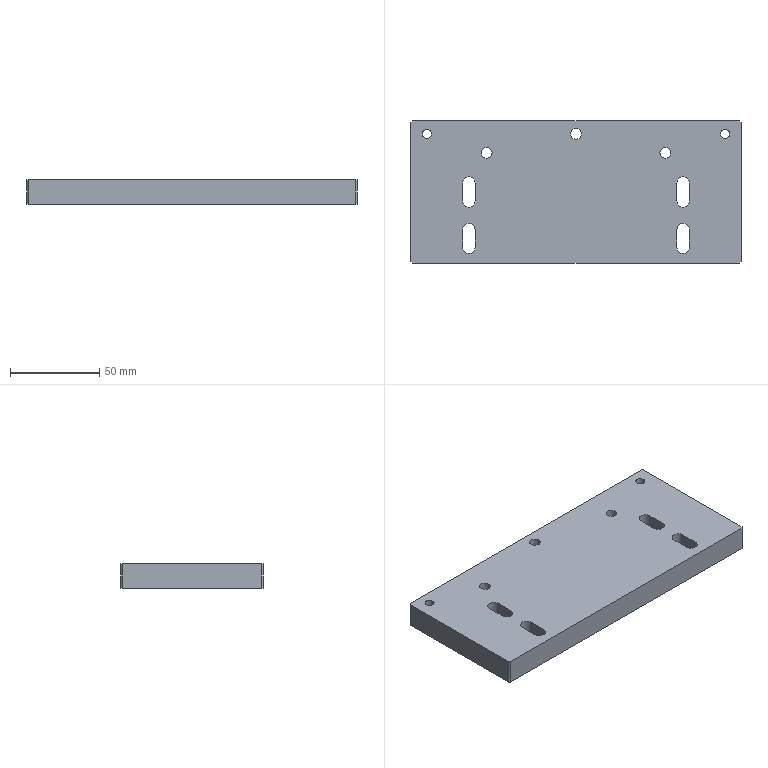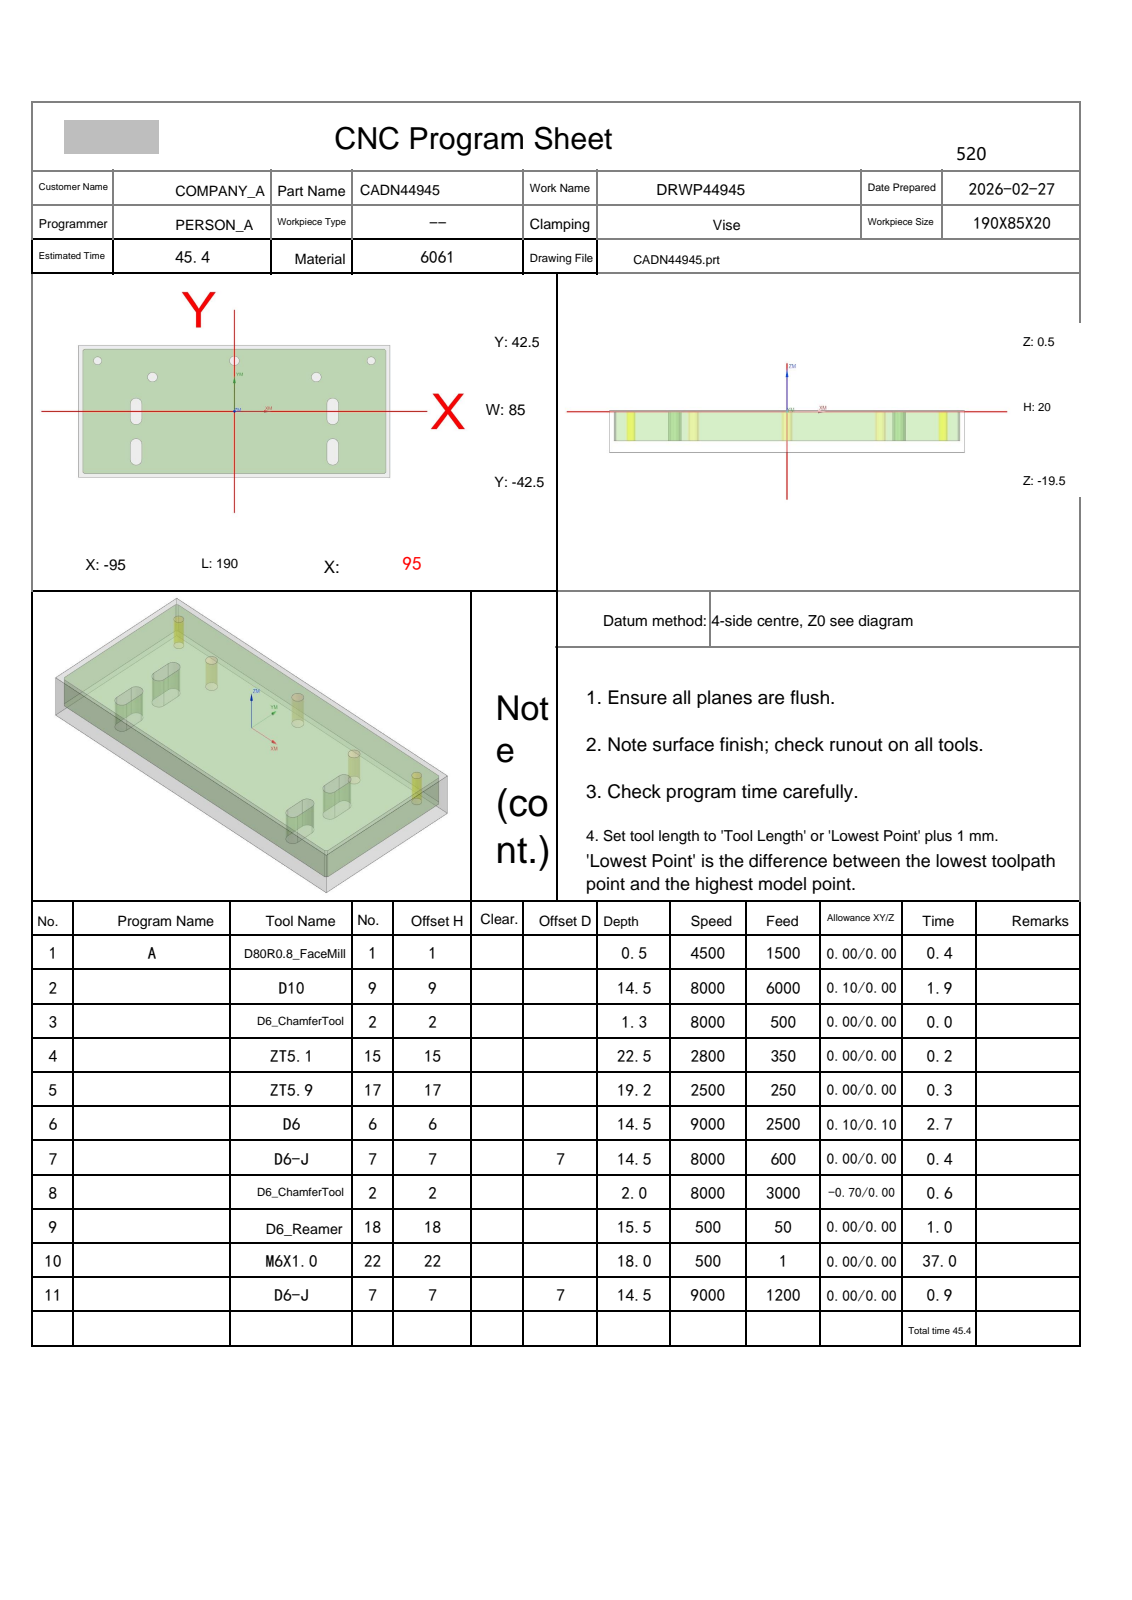NC program | NX | posted by the shop | part box 185 x 80 x 14 mm
Lines 1 to 438 of 2772:
%
O0001
(Machine time: 82.56 MIN)
(===Total Tool:9===)
(T1=D80R0.8-FaceMill D=80.  R=0.8  D-  H01 Z=0.    )
(T9=D10     D=10.  R=0.   D-  H09 Z=-14.  )
(T2=D6_ChamferTool   D=6.   R=0.   D-  H02 Z=-1.5  )
(T15=ZT5.1  D=5.1  DR_a=118 D-  H15 Z=-22.  )
(T17=ZT5.9  D=5.9  DR_a=120 D-  H17 Z=-18.7 )
(T6=D6      D=6.   R=0.   D-  H06 Z=-14.  )
(T7=D6-J    D=6.   R=0.   D7  H07 Z=-14.  )
(T18=D6_Reamer   D=6.   DR_a=180 D-  H18 Z=-15.  )
(T22=M6X1.0 D=5.   DR_a=180 D-  H22 Z=-17.5 )
G80 G90 G17 G49 G40
G91 G28 Z0
M01
N1 T01 M06
(D80R0.8-FaceMill  D=80. R=0.8 H=01 ce=0.00 di=0.00)
G00 G90 G54 X-137.5 Y26.667 M03 S4500
G43 H01 Z50.
M08
Z2.
G01 Z0.0 F1500.
X-132.5
X132.5
Y-26.667
X-132.5
X-137.5
Z2.
G00 Z50.
G91 G28 Z0.0
M05
M09
G91 G28 Z0.0
M01
N2 T09 M06
(D10  D=10. R=0. H=09 ce=0.10 di=0.00)
G00 G90 G54 X0.0 Y-45.1 M03 S8000
G43 H09 Z50.
M08
Z.5
G01 X-91.5 Z.375 F6000.
G02 X-95.106 Y-43.606 Z.37 I0.0 J5.1
G01 X-96.106 Y-42.606 Z.368
G02 X-97.6 Y-39. Z.362 I3.606 J3.606
G01 Y39. Z.256
G02 X-96.106 Y42.606 Z.251 I5.1 J0.0
G01 X-95.106 Y43.606 Z.249
G02 X-93.181 Y44.815 Z.246 I3.606 J-3.606
X-91.5 Y45.1 Z.243 I1.681 J-4.815
G01 X91.5 Z-.006
G02 X95.106 Y43.606 Z-.012 I0.0 J-5.1
G01 X96.106 Y42.606 Z-.014
G02 X97.6 Y39. Z-.019 I-3.606 J-3.606
G01 Y-39. Z-.126
G02 X96.106 Y-42.606 Z-.131 I-5.1 J0.0
G01 X95.106 Y-43.606 Z-.133
G02 X91.5 Y-45.1 Z-.138 I-3.606 J3.606
G01 X-91.5 Z-.388
G02 X-95.106 Y-43.606 Z-.393 I0.0 J5.1
G01 X-96.106 Y-42.606 Z-.395
G02 X-97.6 Y-39. Z-.401 I3.606 J3.606
G01 Y39. Z-.507
G02 X-96.106 Y42.606 Z-.513 I5.1 J0.0
G01 X-95.106 Y43.606 Z-.515
G02 X-93.181 Y44.815 Z-.518 I3.606 J-3.606
X-91.5 Y45.1 Z-.52 I1.681 J-4.815
G01 X91.5 Z-.769
G02 X95.106 Y43.606 Z-.775 I0.0 J-5.1
G01 X96.106 Y42.606 Z-.777
G02 X97.6 Y39. Z-.782 I-3.606 J-3.606
G01 Y-39. Z-.889
G02 X96.106 Y-42.606 Z-.894 I-5.1 J0.0
G01 X95.106 Y-43.606 Z-.896
G02 X91.5 Y-45.1 Z-.902 I-3.606 J3.606
G01 X-91.5 Z-1.151
G02 X-95.106 Y-43.606 Z-1.157 I0.0 J5.1
G01 X-96.106 Y-42.606 Z-1.158
G02 X-97.6 Y-39. Z-1.164 I3.606 J3.606
G01 Y39. Z-1.27
G02 X-96.106 Y42.606 Z-1.276 I5.1 J0.0
G01 X-95.106 Y43.606 Z-1.278
G02 X-93.181 Y44.815 Z-1.281 I3.606 J-3.606
X-91.5 Y45.1 Z-1.283 I1.681 J-4.815
G01 X91.5 Z-1.533
G02 X95.106 Y43.606 Z-1.538 I0.0 J-5.1
G01 X96.106 Y42.606 Z-1.54
G02 X97.6 Y39. Z-1.546 I-3.606 J-3.606
G01 Y-39. Z-1.652
G02 X96.106 Y-42.606 Z-1.657 I-5.1 J0.0
G01 X95.106 Y-43.606 Z-1.659
G02 X91.5 Y-45.1 Z-1.665 I-3.606 J3.606
G01 X-91.5 Z-1.914
G02 X-95.106 Y-43.606 Z-1.92 I0.0 J5.1
G01 X-96.106 Y-42.606 Z-1.922
G02 X-97.6 Y-39. Z-1.927 I3.606 J3.606
G01 Y39. Z-2.033
G02 X-96.106 Y42.606 Z-2.039 I5.1 J0.0
G01 X-95.106 Y43.606 Z-2.041
G02 X-93.181 Y44.815 Z-2.044 I3.606 J-3.606
X-91.5 Y45.1 Z-2.046 I1.681 J-4.815
G01 X91.5 Z-2.296
G02 X95.106 Y43.606 Z-2.301 I0.0 J-5.1
G01 X96.106 Y42.606 Z-2.303
G02 X97.6 Y39. Z-2.309 I-3.606 J-3.606
G01 Y-39. Z-2.415
G02 X96.106 Y-42.606 Z-2.42 I-5.1 J0.0
G01 X95.106 Y-43.606 Z-2.422
G02 X91.5 Y-45.1 Z-2.428 I-3.606 J3.606
G01 X-91.5 Z-2.677
G02 X-95.106 Y-43.606 Z-2.683 I0.0 J5.1
G01 X-96.106 Y-42.606 Z-2.685
G02 X-97.6 Y-39. Z-2.69 I3.606 J3.606
G01 Y39. Z-2.797
G02 X-96.106 Y42.606 Z-2.802 I5.1 J0.0
G01 X-95.106 Y43.606 Z-2.804
G02 X-93.181 Y44.815 Z-2.807 I3.606 J-3.606
X-91.5 Y45.1 Z-2.809 I1.681 J-4.815
G01 X91.5 Z-3.059
G02 X95.106 Y43.606 Z-3.064 I0.0 J-5.1
G01 X96.106 Y42.606 Z-3.066
G02 X97.6 Y39. Z-3.072 I-3.606 J-3.606
G01 Y-39. Z-3.178
G02 X96.106 Y-42.606 Z-3.184 I-5.1 J0.0
G01 X95.106 Y-43.606 Z-3.186
G02 X91.5 Y-45.1 Z-3.191 I-3.606 J3.606
G01 X-91.5 Z-3.441
G02 X-95.106 Y-43.606 Z-3.446 I0.0 J5.1
G01 X-96.106 Y-42.606 Z-3.448
G02 X-97.6 Y-39. Z-3.453 I3.606 J3.606
G01 Y39. Z-3.56
G02 X-96.106 Y42.606 Z-3.565 I5.1 J0.0
G01 X-95.106 Y43.606 Z-3.567
G02 X-93.181 Y44.815 Z-3.57 I3.606 J-3.606
X-91.5 Y45.1 Z-3.573 I1.681 J-4.815
G01 X91.5 Z-3.822
G02 X95.106 Y43.606 Z-3.828 I0.0 J-5.1
G01 X96.106 Y42.606 Z-3.83
G02 X97.6 Y39. Z-3.835 I-3.606 J-3.606
G01 Y-39. Z-3.941
G02 X96.106 Y-42.606 Z-3.947 I-5.1 J0.0
G01 X95.106 Y-43.606 Z-3.949
G02 X91.5 Y-45.1 Z-3.954 I-3.606 J3.606
G01 X-91.5 Z-4.204
G02 X-95.106 Y-43.606 Z-4.209 I0.0 J5.1
G01 X-96.106 Y-42.606 Z-4.211
G02 X-97.6 Y-39. Z-4.217 I3.606 J3.606
G01 Y39. Z-4.323
G02 X-96.106 Y42.606 Z-4.328 I5.1 J0.0
G01 X-95.106 Y43.606 Z-4.33
G02 X-93.181 Y44.815 Z-4.333 I3.606 J-3.606
X-91.5 Y45.1 Z-4.336 I1.681 J-4.815
G01 X91.5 Z-4.585
G02 X95.106 Y43.606 Z-4.591 I0.0 J-5.1
G01 X96.106 Y42.606 Z-4.593
G02 X97.6 Y39. Z-4.598 I-3.606 J-3.606
G01 Y-39. Z-4.704
G02 X96.106 Y-42.606 Z-4.71 I-5.1 J0.0
G01 X95.106 Y-43.606 Z-4.712
G02 X91.5 Y-45.1 Z-4.717 I-3.606 J3.606
G01 X-91.5 Z-4.967
G02 X-95.106 Y-43.606 Z-4.972 I0.0 J5.1
G01 X-96.106 Y-42.606 Z-4.974
G02 X-97.6 Y-39. Z-4.98 I3.606 J3.606
G01 Y39. Z-5.086
G02 X-96.106 Y42.606 Z-5.092 I5.1 J0.0
G01 X-95.106 Y43.606 Z-5.093
G02 X-93.181 Y44.815 Z-5.097 I3.606 J-3.606
X-91.5 Y45.1 Z-5.099 I1.681 J-4.815
G01 X91.5 Z-5.348
G02 X95.106 Y43.606 Z-5.354 I0.0 J-5.1
G01 X96.106 Y42.606 Z-5.356
G02 X97.6 Y39. Z-5.361 I-3.606 J-3.606
G01 Y-39. Z-5.468
G02 X96.106 Y-42.606 Z-5.473 I-5.1 J0.0
G01 X95.106 Y-43.606 Z-5.475
G02 X91.5 Y-45.1 Z-5.481 I-3.606 J3.606
G01 X-91.5 Z-5.73
G02 X-95.106 Y-43.606 Z-5.735 I0.0 J5.1
G01 X-96.106 Y-42.606 Z-5.737
G02 X-97.6 Y-39. Z-5.743 I3.606 J3.606
G01 Y39. Z-5.849
G02 X-96.106 Y42.606 Z-5.855 I5.1 J0.0
G01 X-95.106 Y43.606 Z-5.857
G02 X-93.181 Y44.815 Z-5.86 I3.606 J-3.606
X-91.5 Y45.1 Z-5.862 I1.681 J-4.815
G01 X91.5 Z-6.112
G02 X95.106 Y43.606 Z-6.117 I0.0 J-5.1
G01 X96.106 Y42.606 Z-6.119
G02 X97.6 Y39. Z-6.124 I-3.606 J-3.606
G01 Y-39. Z-6.231
G02 X96.106 Y-42.606 Z-6.236 I-5.1 J0.0
G01 X95.106 Y-43.606 Z-6.238
G02 X91.5 Y-45.1 Z-6.244 I-3.606 J3.606
G01 X-91.5 Z-6.493
G02 X-95.106 Y-43.606 Z-6.499 I0.0 J5.1
G01 X-96.106 Y-42.606 Z-6.501
G02 X-97.6 Y-39. Z-6.506 I3.606 J3.606
G01 Y39. Z-6.612
G02 X-96.106 Y42.606 Z-6.618 I5.1 J0.0
G01 X-95.106 Y43.606 Z-6.62
G02 X-93.181 Y44.815 Z-6.623 I3.606 J-3.606
X-91.5 Y45.1 Z-6.625 I1.681 J-4.815
G01 X91.5 Z-6.875
G02 X95.106 Y43.606 Z-6.88 I0.0 J-5.1
G01 X96.106 Y42.606 Z-6.882
G02 X97.6 Y39. Z-6.888 I-3.606 J-3.606
G01 Y-39. Z-6.994
G02 X96.106 Y-42.606 Z-6.999 I-5.1 J0.0
G01 X95.106 Y-43.606 Z-7.001
G02 X91.5 Y-45.1 Z-7.007 I-3.606 J3.606
G01 X-91.5 Z-7.256
G02 X-95.106 Y-43.606 Z-7.262 I0.0 J5.1
G01 X-96.106 Y-42.606 Z-7.264
G02 X-97.6 Y-39. Z-7.269 I3.606 J3.606
G01 Y39. Z-7.376
G02 X-96.106 Y42.606 Z-7.381 I5.1 J0.0
G01 X-95.106 Y43.606 Z-7.383
G02 X-93.181 Y44.815 Z-7.386 I3.606 J-3.606
X-91.5 Y45.1 Z-7.388 I1.681 J-4.815
G01 X91.5 Z-7.638
G02 X95.106 Y43.606 Z-7.643 I0.0 J-5.1
G01 X96.106 Y42.606 Z-7.645
G02 X97.6 Y39. Z-7.651 I-3.606 J-3.606
G01 Y-39. Z-7.757
G02 X96.106 Y-42.606 Z-7.763 I-5.1 J0.0
G01 X95.106 Y-43.606 Z-7.765
G02 X91.5 Y-45.1 Z-7.77 I-3.606 J3.606
G01 X-91.5 Z-8.019
G02 X-95.106 Y-43.606 Z-8.025 I0.0 J5.1
G01 X-96.106 Y-42.606 Z-8.027
G02 X-97.6 Y-39. Z-8.032 I3.606 J3.606
G01 Y39. Z-8.139
G02 X-96.106 Y42.606 Z-8.144 I5.1 J0.0
G01 X-95.106 Y43.606 Z-8.146
G02 X-93.181 Y44.815 Z-8.149 I3.606 J-3.606
X-91.5 Y45.1 Z-8.152 I1.681 J-4.815
G01 X91.5 Z-8.401
G02 X95.106 Y43.606 Z-8.407 I0.0 J-5.1
G01 X96.106 Y42.606 Z-8.408
G02 X97.6 Y39. Z-8.414 I-3.606 J-3.606
G01 Y-39. Z-8.52
G02 X96.106 Y-42.606 Z-8.526 I-5.1 J0.0
G01 X95.106 Y-43.606 Z-8.528
G02 X91.5 Y-45.1 Z-8.533 I-3.606 J3.606
G01 X-91.5 Z-8.783
G02 X-95.106 Y-43.606 Z-8.788 I0.0 J5.1
G01 X-96.106 Y-42.606 Z-8.79
G02 X-97.6 Y-39. Z-8.796 I3.606 J3.606
G01 Y39. Z-8.902
G02 X-96.106 Y42.606 Z-8.907 I5.1 J0.0
G01 X-95.106 Y43.606 Z-8.909
G02 X-93.181 Y44.815 Z-8.912 I3.606 J-3.606
X-91.5 Y45.1 Z-8.915 I1.681 J-4.815
G01 X91.5 Z-9.164
G02 X95.106 Y43.606 Z-9.17 I0.0 J-5.1
G01 X96.106 Y42.606 Z-9.172
G02 X97.6 Y39. Z-9.177 I-3.606 J-3.606
G01 Y-39. Z-9.283
G02 X96.106 Y-42.606 Z-9.289 I-5.1 J0.0
G01 X95.106 Y-43.606 Z-9.291
G02 X91.5 Y-45.1 Z-9.296 I-3.606 J3.606
G01 X-91.5 Z-9.546
G02 X-95.106 Y-43.606 Z-9.551 I0.0 J5.1
G01 X-96.106 Y-42.606 Z-9.553
G02 X-97.6 Y-39. Z-9.559 I3.606 J3.606
G01 Y39. Z-9.665
G02 X-96.106 Y42.606 Z-9.67 I5.1 J0.0
G01 X-95.106 Y43.606 Z-9.672
G02 X-93.181 Y44.815 Z-9.676 I3.606 J-3.606
X-91.5 Y45.1 Z-9.678 I1.681 J-4.815
G01 X91.5 Z-9.927
G02 X95.106 Y43.606 Z-9.933 I0.0 J-5.1
G01 X96.106 Y42.606 Z-9.935
G02 X97.6 Y39. Z-9.94 I-3.606 J-3.606
G01 Y-39. Z-10.047
G02 X96.106 Y-42.606 Z-10.052 I-5.1 J0.0
G01 X95.106 Y-43.606 Z-10.054
G02 X91.5 Y-45.1 Z-10.059 I-3.606 J3.606
G01 X-91.5 Z-10.309
G02 X-95.106 Y-43.606 Z-10.314 I0.0 J5.1
G01 X-96.106 Y-42.606 Z-10.316
G02 X-97.6 Y-39. Z-10.322 I3.606 J3.606
G01 Y39. Z-10.428
G02 X-96.106 Y42.606 Z-10.434 I5.1 J0.0
G01 X-95.106 Y43.606 Z-10.436
G02 X-93.181 Y44.815 Z-10.439 I3.606 J-3.606
X-91.5 Y45.1 Z-10.441 I1.681 J-4.815
G01 X91.5 Z-10.691
G02 X95.106 Y43.606 Z-10.696 I0.0 J-5.1
G01 X96.106 Y42.606 Z-10.698
G02 X97.6 Y39. Z-10.703 I-3.606 J-3.606
G01 Y-39. Z-10.81
G02 X96.106 Y-42.606 Z-10.815 I-5.1 J0.0
G01 X95.106 Y-43.606 Z-10.817
G02 X91.5 Y-45.1 Z-10.823 I-3.606 J3.606
G01 X-91.5 Z-11.072
G02 X-95.106 Y-43.606 Z-11.078 I0.0 J5.1
G01 X-96.106 Y-42.606 Z-11.08
G02 X-97.6 Y-39. Z-11.085 I3.606 J3.606
G01 Y39. Z-11.191
G02 X-96.106 Y42.606 Z-11.197 I5.1 J0.0
G01 X-95.106 Y43.606 Z-11.199
G02 X-93.181 Y44.815 Z-11.202 I3.606 J-3.606
X-91.5 Y45.1 Z-11.204 I1.681 J-4.815
G01 X91.5 Z-11.454
G02 X95.106 Y43.606 Z-11.459 I0.0 J-5.1
G01 X96.106 Y42.606 Z-11.461
G02 X97.6 Y39. Z-11.467 I-3.606 J-3.606
G01 Y-39. Z-11.573
G02 X96.106 Y-42.606 Z-11.578 I-5.1 J0.0
G01 X95.106 Y-43.606 Z-11.58
G02 X91.5 Y-45.1 Z-11.586 I-3.606 J3.606
G01 X-91.5 Z-11.835
G02 X-95.106 Y-43.606 Z-11.841 I0.0 J5.1
G01 X-96.106 Y-42.606 Z-11.843
G02 X-97.6 Y-39. Z-11.848 I3.606 J3.606
G01 Y39. Z-11.954
G02 X-96.106 Y42.606 Z-11.96 I5.1 J0.0
G01 X-95.106 Y43.606 Z-11.962
G02 X-93.181 Y44.815 Z-11.965 I3.606 J-3.606
X-91.5 Y45.1 Z-11.967 I1.681 J-4.815
G01 X91.5 Z-12.217
G02 X95.106 Y43.606 Z-12.222 I0.0 J-5.1
G01 X96.106 Y42.606 Z-12.224
G02 X97.6 Y39. Z-12.23 I-3.606 J-3.606
G01 Y-39. Z-12.336
G02 X96.106 Y-42.606 Z-12.342 I-5.1 J0.0
G01 X95.106 Y-43.606 Z-12.343
G02 X91.5 Y-45.1 Z-12.349 I-3.606 J3.606
G01 X-91.5 Z-12.598
G02 X-95.106 Y-43.606 Z-12.604 I0.0 J5.1
G01 X-96.106 Y-42.606 Z-12.606
G02 X-97.6 Y-39. Z-12.611 I3.606 J3.606
G01 Y39. Z-12.718
G02 X-96.106 Y42.606 Z-12.723 I5.1 J0.0
G01 X-95.106 Y43.606 Z-12.725
G02 X-93.181 Y44.815 Z-12.728 I3.606 J-3.606
X-91.5 Y45.1 Z-12.731 I1.681 J-4.815
G01 X91.5 Z-12.98
G02 X95.106 Y43.606 Z-12.985 I0.0 J-5.1
G01 X96.106 Y42.606 Z-12.987
G02 X97.6 Y39. Z-12.993 I-3.606 J-3.606
G01 Y-39. Z-13.099
G02 X96.106 Y-42.606 Z-13.105 I-5.1 J0.0
G01 X95.106 Y-43.606 Z-13.107
G02 X91.5 Y-45.1 Z-13.112 I-3.606 J3.606
G01 X-91.5 Z-13.362
G02 X-95.106 Y-43.606 Z-13.367 I0.0 J5.1
G01 X-96.106 Y-42.606 Z-13.369
G02 X-97.6 Y-39. Z-13.374 I3.606 J3.606
G01 Y39. Z-13.481
G02 X-96.106 Y42.606 Z-13.486 I5.1 J0.0
G01 X-95.106 Y43.606 Z-13.488
G02 X-93.181 Y44.815 Z-13.491 I3.606 J-3.606
X-91.5 Y45.1 Z-13.494 I1.681 J-4.815
G01 X91.5 Z-13.743
G02 X95.106 Y43.606 Z-13.749 I0.0 J-5.1
G01 X96.106 Y42.606 Z-13.751
G02 X97.6 Y39. Z-13.756 I-3.606 J-3.606
G01 Y-39. Z-13.862
G02 X96.106 Y-42.606 Z-13.868 I-5.1 J0.0
G01 X95.106 Y-43.606 Z-13.87
G02 X91.5 Y-45.1 Z-13.875 I-3.606 J3.606
G01 X0.0 Z-14.
X-91.5
G02 X-95.106 Y-43.606 I0.0 J5.1
G01 X-96.106 Y-42.606
G02 X-97.6 Y-39. I3.606 J3.606
G01 Y39.
G02 X-96.106 Y42.606 I5.1 J0.0
G01 X-95.106 Y43.606
G02 X-91.5 Y45.1 I3.606 J-3.606
G01 X91.5
G02 X95.106 Y43.606 I0.0 J-5.1
G01 X96.106 Y42.606
G02 X97.6 Y39. I-3.606 J-3.606
G01 Y-39.
G02 X96.106 Y-42.606 I-5.1 J0.0
G01 X95.106 Y-43.606
G02 X91.5 Y-45.1 I-3.606 J3.606
G01 X0.0
X-.5
Z-13.
G00 Z50.
G91 G28 Z0.0
M05
M09
G91 G28 Z0.0
M01
N3 T02 M06
(D6_ChamferTool  D=6. R=0. H=02 ce=0.00 di=0.00)
G00 G90 G54 X-83.5 Y32.5 M03 S8000
G43 H02 Z50.
M08
G98 G81 X-83.5 Y32.5 Z-.8 R1. F500.
X-50. Y22.
X0.0 Y32.5
X50. Y22.
X83.5 Y32.5
G80
G00 Z50.
G91 G28 Z0.0
M05
M09
G91 G28 Z0.0
M01
N4 T15 M06
(ZT5.1 D=5.1 DR_a=118 H=15)
G00 G90 G54 X-83.5 Y32.5 M03 S2800
G43 H15 Z50.
M08
G98 G83 X-83.5 Y32.5 Z-22. R1. F350. Q3.
X83.5
G80
G00 Z50.
G91 G28 Z0.0
M05
M09
G91 G28 Z0.0
M01
N5 T17 M06
(ZT5.9 D=5.9 DR_a=120 H=17)
G00 G90 G54 X50. Y22. M03 S2500
G43 H17 Z50.
M08
G98 G83 X50. Y22. Z-18.703 R1. F250. Q2.
X0.0 Y32.5
X-50. Y22.
G80
G00 Z50.
G91 G28 Z0.0
M05
M09
G91 G28 Z0.0
M01